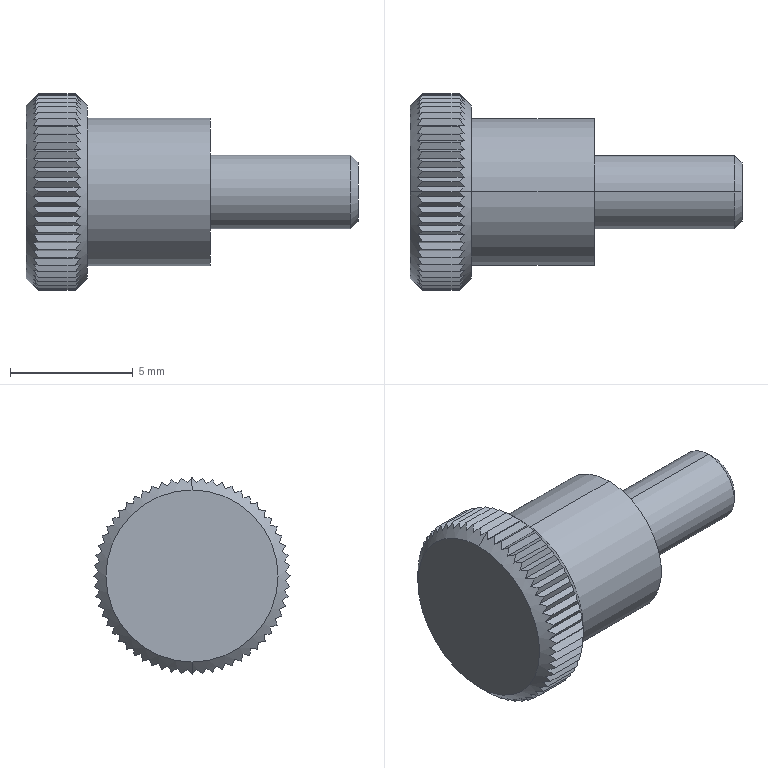Part | SolidWorks | features MBimport 1 | 1 solid | 134 faces | box 13.5 x 8 x 8 mm | volume 298.871 mm3 | plane 124 | cone 6 | cylinder 4 | commonest cylinder face diameters 3 x2 6 x2